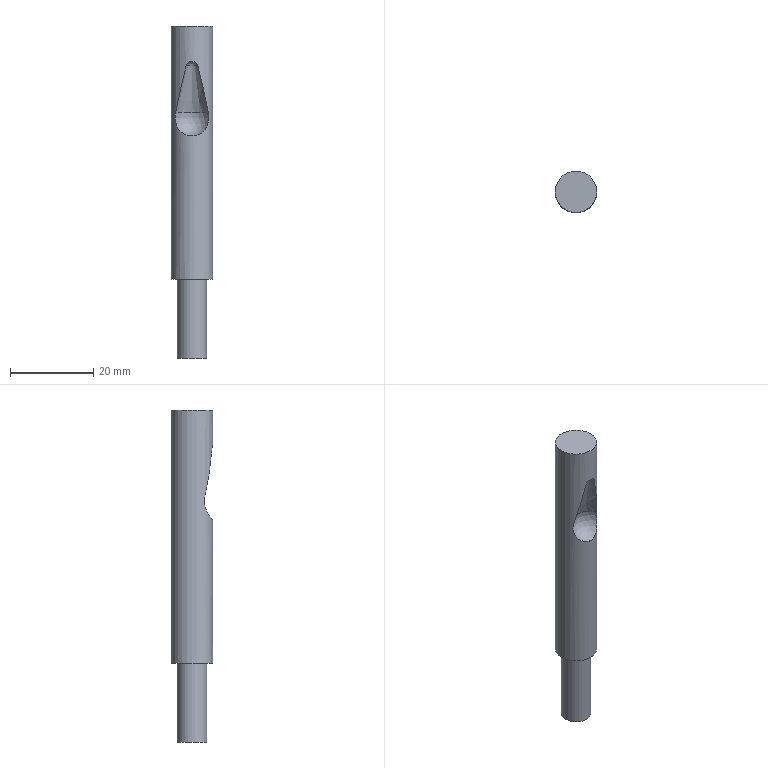Part | NX | features solid 2 | 1 solid | 8 faces | volume 5295 mm3 | plane 3 | cylinder 2 | sphere 2 | cone 1 | commonest cylinder face diameters 7.1 x1 10 x1
STEP:
#1=CARTESIAN_POINT('',(-1301.921,535.139,81.125));
#2=VERTEX_POINT('',#1);
#3=CARTESIAN_POINT('',(-1299.436,533.451,92.375));
#4=VERTEX_POINT('',#3);
#5=CARTESIAN_POINT('',(-1301.921,535.139,81.125));
#6=CARTESIAN_POINT('',(-1301.256,534.298,84.863));
#7=CARTESIAN_POINT('',(-1300.377,533.733,88.613));
#8=CARTESIAN_POINT('',(-1299.436,533.451,92.375));
#9=B_SPLINE_CURVE_WITH_KNOTS('',3,(#5,#6,#7,#8),.UNSPECIFIED.,.F.,.F.,(4,4),(0.000000208,0.01165),.UNSPECIFIED.);
#10=EDGE_CURVE('',#2,#4,#9,.T.);
#11=ORIENTED_EDGE('',*,*,#10,.T.);
#12=CARTESIAN_POINT('',(-1296.562,533.451,92.375));
#13=VERTEX_POINT('',#12);
#14=CARTESIAN_POINT('',(-1299.436,533.451,92.375));
#15=CARTESIAN_POINT('',(-1299.275,533.403,93.02));
#16=CARTESIAN_POINT('',(-1298.001,533.078,93.98));
#17=CARTESIAN_POINT('',(-1296.723,533.403,93.02));
#18=CARTESIAN_POINT('',(-1296.562,533.451,92.375));
#19=B_SPLINE_CURVE_WITH_KNOTS('',3,(#14,#15,#16,#17,#18),.UNSPECIFIED.,.F.,.F.,(4,1,4),(0.000000204,0.001971,0.003941),.UNSPECIFIED.);
#20=EDGE_CURVE('',#4,#13,#19,.T.);
#21=ORIENTED_EDGE('',*,*,#20,.T.);
#22=CARTESIAN_POINT('',(-1294.077,535.139,81.125));
#23=VERTEX_POINT('',#22);
#24=CARTESIAN_POINT('',(-1296.562,533.451,92.375));
#25=CARTESIAN_POINT('',(-1295.622,533.733,88.611));
#26=CARTESIAN_POINT('',(-1294.743,534.297,84.865));
#27=CARTESIAN_POINT('',(-1294.077,535.139,81.125));
#28=B_SPLINE_CURVE_WITH_KNOTS('',3,(#24,#25,#26,#27),.UNSPECIFIED.,.F.,.F.,(4,4),(0.000000207,0.01167),.UNSPECIFIED.);
#29=EDGE_CURVE('',#13,#23,#28,.T.);
#30=ORIENTED_EDGE('',*,*,#29,.T.);
#31=CARTESIAN_POINT('',(-1294.077,535.139,81.125));
#32=CARTESIAN_POINT('',(-1293.958,535.29,80.454));
#33=CARTESIAN_POINT('',(-1293.939,535.316,79.034));
#34=CARTESIAN_POINT('',(-1294.552,534.535,77.139));
#35=CARTESIAN_POINT('',(-1295.928,533.554,75.833));
#36=CARTESIAN_POINT('',(-1297.985,533.085,75.336));
#37=CARTESIAN_POINT('',(-1300.062,533.547,75.825));
#38=CARTESIAN_POINT('',(-1301.447,534.535,77.139));
#39=CARTESIAN_POINT('',(-1302.059,535.314,79.026));
#40=CARTESIAN_POINT('',(-1302.041,535.29,80.453));
#41=CARTESIAN_POINT('',(-1301.921,535.139,81.125));
#42=B_SPLINE_CURVE_WITH_KNOTS('',3,(#31,#32,#33,#34,#35,#36,#37,#38,#39,#40,#41),.UNSPECIFIED.,.F.,.F.,(4,1,1,1,1,1,1,1,4),(0.000000205,0.002065,0.00413,0.006195,0.00826,0.01033,0.01239,0.01446,0.01652),.UNSPECIFIED.);
#43=EDGE_CURVE('',#23,#2,#42,.T.);
#44=ORIENTED_EDGE('',*,*,#43,.T.);
#45=EDGE_LOOP('',(#11,#21,#30,#44));
#46=FACE_BOUND('',#45,.T.);
#47=CARTESIAN_POINT('',(-1302.999,538.24,102.));
#48=VERTEX_POINT('',#47);
#49=CARTESIAN_POINT('',(-1297.999,538.24,102.));
#50=DIRECTION('',(0.,0.,1.));
#51=DIRECTION('',(-1.,0.,0.));
#52=AXIS2_PLACEMENT_3D('',#49,#50,#51);
#53=CIRCLE('',#52,5.);
#54=EDGE_CURVE('',#48,#48,#53,.T.);
#55=ORIENTED_EDGE('',*,*,#54,.F.);
#56=EDGE_LOOP('',(#55));
#57=FACE_BOUND('',#56,.T.);
#58=CARTESIAN_POINT('',(-1292.999,538.24,41.));
#59=VERTEX_POINT('',#58);
#60=CARTESIAN_POINT('',(-1297.999,538.24,41.));
#61=DIRECTION('',(0.,0.,1.));
#62=DIRECTION('',(1.,0.,0.));
#63=AXIS2_PLACEMENT_3D('',#60,#61,#62);
#64=CIRCLE('',#63,5.);
#65=EDGE_CURVE('',#59,#59,#64,.T.);
#66=ORIENTED_EDGE('',*,*,#65,.T.);
#67=EDGE_LOOP('',(#66));
#68=FACE_BOUND('',#67,.T.);
#69=CARTESIAN_POINT('',(-1297.999,538.24,102.));
#70=DIRECTION('',(0.,0.,-1.));
#71=DIRECTION('',(1.,0.,0.));
#72=AXIS2_PLACEMENT_3D('',#69,#70,#71);
#73=CYLINDRICAL_SURFACE('',#72,5.);
#74=ADVANCED_FACE('',(#46,#57,#68),#73,.T.);
#75=ORIENTED_EDGE('',*,*,#54,.T.);
#76=EDGE_LOOP('',(#75));
#77=FACE_BOUND('',#76,.T.);
#78=CARTESIAN_POINT('',(-1297.999,538.24,102.));
#79=DIRECTION('',(0.,0.,1.));
#80=DIRECTION('',(-1.,0.,0.));
#81=AXIS2_PLACEMENT_3D('',#78,#79,#80);
#82=PLANE('',#81);
#83=ADVANCED_FACE('',(#77),#82,.T.);
#84=CARTESIAN_POINT('',(-1294.449,538.24,41.));
#85=VERTEX_POINT('',#84);
#86=CARTESIAN_POINT('',(-1297.999,538.24,41.));
#87=DIRECTION('',(0.,0.,1.));
#88=DIRECTION('',(1.,0.,0.));
#89=AXIS2_PLACEMENT_3D('',#86,#87,#88);
#90=CIRCLE('',#89,3.55);
#91=EDGE_CURVE('',#85,#85,#90,.T.);
#92=ORIENTED_EDGE('',*,*,#91,.T.);
#93=EDGE_LOOP('',(#92));
#94=FACE_BOUND('',#93,.T.);
#95=ORIENTED_EDGE('',*,*,#65,.F.);
#96=EDGE_LOOP('',(#95));
#97=FACE_BOUND('',#96,.T.);
#98=CARTESIAN_POINT('',(-1297.999,538.24,41.));
#99=DIRECTION('',(0.,0.,1.));
#100=DIRECTION('',(-1.,0.,0.));
#101=AXIS2_PLACEMENT_3D('',#98,#99,#100);
#102=PLANE('',#101);
#103=ADVANCED_FACE('',(#94,#97),#102,.F.);
#104=CARTESIAN_POINT('',(-1294.449,538.24,22.));
#105=VERTEX_POINT('',#104);
#106=CARTESIAN_POINT('',(-1297.999,538.24,22.));
#107=DIRECTION('',(0.,0.,1.));
#108=DIRECTION('',(1.,0.,0.));
#109=AXIS2_PLACEMENT_3D('',#106,#107,#108);
#110=CIRCLE('',#109,3.55);
#111=EDGE_CURVE('',#105,#105,#110,.T.);
#112=ORIENTED_EDGE('',*,*,#111,.T.);
#113=EDGE_LOOP('',(#112));
#114=FACE_BOUND('',#113,.T.);
#115=ORIENTED_EDGE('',*,*,#91,.F.);
#116=EDGE_LOOP('',(#115));
#117=FACE_BOUND('',#116,.T.);
#118=CARTESIAN_POINT('',(-1297.999,538.24,12.));
#119=DIRECTION('',(0.,0.,1.));
#120=DIRECTION('',(-1.,0.,0.));
#121=AXIS2_PLACEMENT_3D('',#118,#119,#120);
#122=CYLINDRICAL_SURFACE('',#121,3.55);
#123=ADVANCED_FACE('',(#114,#117),#122,.T.);
#124=ORIENTED_EDGE('',*,*,#111,.F.);
#125=EDGE_LOOP('',(#124));
#126=FACE_BOUND('',#125,.T.);
#127=CARTESIAN_POINT('',(-1297.999,538.24,22.));
#128=DIRECTION('',(0.,0.,1.));
#129=DIRECTION('',(-1.,0.,0.));
#130=AXIS2_PLACEMENT_3D('',#127,#128,#129);
#131=PLANE('',#130);
#132=ADVANCED_FACE('',(#126),#131,.F.);
#133=CARTESIAN_POINT('',(-1297.999,533.24,81.125));
#134=DIRECTION('',(0.,0.,-1.));
#135=DIRECTION('',(1.,0.,0.));
#136=AXIS2_PLACEMENT_3D('',#133,#134,#135);
#137=CIRCLE('',#136,4.357);
#138=EDGE_CURVE('',#2,#23,#137,.T.);
#139=ORIENTED_EDGE('',*,*,#138,.F.);
#140=ORIENTED_EDGE('',*,*,#43,.F.);
#141=EDGE_LOOP('',(#139,#140));
#142=FACE_BOUND('',#141,.T.);
#143=CARTESIAN_POINT('',(-1297.999,533.24,80.));
#144=DIRECTION('',(0.,0.,-1.));
#145=DIRECTION('',(1.,0.,0.));
#146=AXIS2_PLACEMENT_3D('',#143,#144,#145);
#147=SPHERICAL_SURFACE('',#146,4.5);
#148=ADVANCED_FACE('',(#142),#147,.F.);
#149=CARTESIAN_POINT('',(-1297.999,533.24,92.375));
#150=DIRECTION('',(0.,0.,-1.));
#151=DIRECTION('',(1.,0.,0.));
#152=AXIS2_PLACEMENT_3D('',#149,#150,#151);
#153=CIRCLE('',#152,1.452);
#154=EDGE_CURVE('',#4,#13,#153,.T.);
#155=ORIENTED_EDGE('',*,*,#154,.F.);
#156=ORIENTED_EDGE('',*,*,#10,.F.);
#157=ORIENTED_EDGE('',*,*,#138,.T.);
#158=ORIENTED_EDGE('',*,*,#29,.F.);
#159=EDGE_LOOP('',(#155,#156,#157,#158));
#160=FACE_BOUND('',#159,.T.);
#161=CARTESIAN_POINT('',(-1297.999,533.24,81.125));
#162=DIRECTION('',(0.,0.,-1.));
#163=DIRECTION('',(1.,0.,0.));
#164=AXIS2_PLACEMENT_3D('',#161,#162,#163);
#165=CONICAL_SURFACE('',#164,4.357,0.2527);
#166=ADVANCED_FACE('',(#160),#165,.F.);
#167=ORIENTED_EDGE('',*,*,#154,.T.);
#168=ORIENTED_EDGE('',*,*,#20,.F.);
#169=EDGE_LOOP('',(#167,#168));
#170=FACE_BOUND('',#169,.T.);
#171=CARTESIAN_POINT('',(-1297.999,533.24,92.));
#172=DIRECTION('',(0.,0.,-1.));
#173=DIRECTION('',(-1.,0.,0.));
#174=AXIS2_PLACEMENT_3D('',#171,#172,#173);
#175=SPHERICAL_SURFACE('',#174,1.5);
#176=ADVANCED_FACE('',(#170),#175,.F.);
#177=CLOSED_SHELL('',(#74,#83,#103,#123,#132,#148,#166,#176));
#178=MANIFOLD_SOLID_BREP('',#177);
#179=(LENGTH_UNIT()NAMED_UNIT(*)SI_UNIT(.MILLI.,.METRE.));
#180=UNCERTAINTY_MEASURE_WITH_UNIT(LENGTH_MEASURE(0.0508),#179,'','');
#181=(NAMED_UNIT(*)PLANE_ANGLE_UNIT()SI_UNIT($,.RADIAN.));
#182=(NAMED_UNIT(*)SI_UNIT($,.STERADIAN.)SOLID_ANGLE_UNIT());
#183=(GEOMETRIC_REPRESENTATION_CONTEXT(3)GLOBAL_UNCERTAINTY_ASSIGNED_CONTEXT((#180))GLOBAL_UNIT_ASSIGNED_CONTEXT((#179,#181,#182))REPRESENTATION_CONTEXT('',''));
#184=ADVANCED_BREP_SHAPE_REPRESENTATION('',(#178),#183);